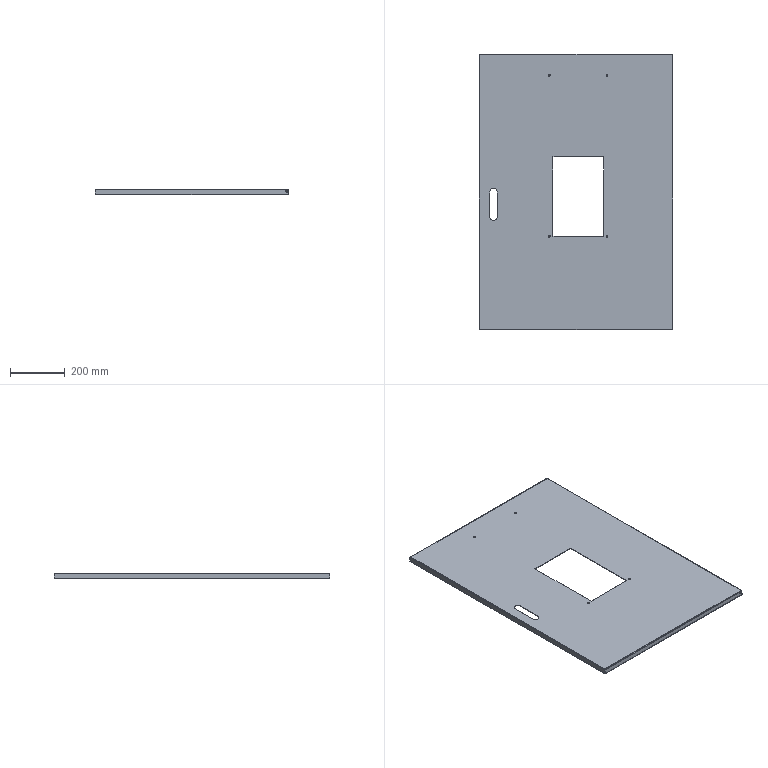Part | STEP file | Electrical Cabinet Door | 1 solid | 114 faces | box 708 x 1006 x 21 mm | volume 1538935 mm3 | plane 68 | cylinder 30 | spline 16 | commonest cylinder face diameters 1 x8 5 x8 6.5 x8 7 x4 27 x2